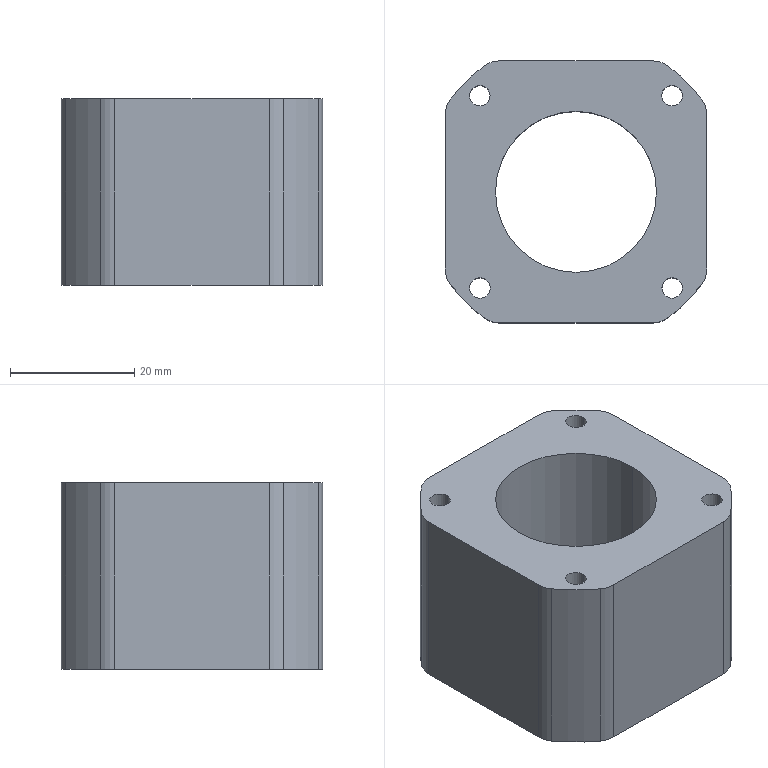Part | SolidWorks | features BaseBody 1 | 1 solid | 28 faces | box 42.13 x 42.13 x 30 mm | volume 33535 mm3 | cylinder 22 | plane 6 | commonest cylinder face diameters 3.3 x8 8 x8 50.215 x4 25.915 x2
STEP:
#1=CARTESIAN_POINT('',(-13.83,15.466,0.));
#2=VERTEX_POINT('',#1);
#3=CARTESIAN_POINT('',(-17.13,15.466,0.));
#4=VERTEX_POINT('',#3);
#5=CARTESIAN_POINT('',(-15.48,15.466,0.));
#6=DIRECTION('',(0.,0.,-1.));
#7=DIRECTION('',(1.,0.,0.));
#8=AXIS2_PLACEMENT_3D('',#5,#6,#7);
#9=CIRCLE('',#8,1.65);
#10=EDGE_CURVE('',#2,#4,#9,.T.);
#11=ORIENTED_EDGE('',*,*,#10,.T.);
#12=CARTESIAN_POINT('',(-17.13,15.466,30.));
#13=VERTEX_POINT('',#12);
#14=CARTESIAN_POINT('',(-17.13,15.466,0.));
#15=DIRECTION('',(0.,0.,1.));
#16=VECTOR('',#15,1000.);
#17=LINE('',#14,#16);
#18=EDGE_CURVE('',#4,#13,#17,.T.);
#19=ORIENTED_EDGE('',*,*,#18,.T.);
#20=CARTESIAN_POINT('',(-13.83,15.466,30.));
#21=VERTEX_POINT('',#20);
#22=CARTESIAN_POINT('',(-15.48,15.466,30.));
#23=DIRECTION('',(0.,0.,1.));
#24=DIRECTION('',(1.,0.,0.));
#25=AXIS2_PLACEMENT_3D('',#22,#23,#24);
#26=CIRCLE('',#25,1.65);
#27=EDGE_CURVE('',#13,#21,#26,.T.);
#28=ORIENTED_EDGE('',*,*,#27,.T.);
#29=CARTESIAN_POINT('',(-13.83,15.466,0.));
#30=DIRECTION('',(0.,0.,1.));
#31=VECTOR('',#30,1000.);
#32=LINE('',#29,#31);
#33=EDGE_CURVE('',#2,#21,#32,.T.);
#34=ORIENTED_EDGE('',*,*,#33,.F.);
#35=EDGE_LOOP('',(#11,#19,#28,#34));
#36=FACE_OUTER_BOUND('',#35,.T.);
#37=CARTESIAN_POINT('',(-15.48,15.466,0.));
#38=DIRECTION('',(0.,0.,1.));
#39=DIRECTION('',(1.,0.,0.));
#40=AXIS2_PLACEMENT_3D('',#37,#38,#39);
#41=CYLINDRICAL_SURFACE('',#40,1.65);
#42=ADVANCED_FACE('',(#36),#41,.F.);
#43=CARTESIAN_POINT('',(12.957,0.,0.));
#44=VERTEX_POINT('',#43);
#45=CARTESIAN_POINT('',(-12.957,0.,0.));
#46=VERTEX_POINT('',#45);
#47=CARTESIAN_POINT('',(0.,0.,0.));
#48=DIRECTION('',(0.,0.,-1.));
#49=DIRECTION('',(1.,0.,0.));
#50=AXIS2_PLACEMENT_3D('',#47,#48,#49);
#51=CIRCLE('',#50,12.957);
#52=EDGE_CURVE('',#44,#46,#51,.T.);
#53=ORIENTED_EDGE('',*,*,#52,.T.);
#54=CARTESIAN_POINT('',(-12.957,0.,30.));
#55=VERTEX_POINT('',#54);
#56=CARTESIAN_POINT('',(-12.957,0.,0.));
#57=DIRECTION('',(0.,0.,1.));
#58=VECTOR('',#57,1000.);
#59=LINE('',#56,#58);
#60=EDGE_CURVE('',#46,#55,#59,.T.);
#61=ORIENTED_EDGE('',*,*,#60,.T.);
#62=CARTESIAN_POINT('',(12.957,0.,30.));
#63=VERTEX_POINT('',#62);
#64=CARTESIAN_POINT('',(0.,0.,30.));
#65=DIRECTION('',(0.,0.,-1.));
#66=DIRECTION('',(1.,0.,0.));
#67=AXIS2_PLACEMENT_3D('',#64,#65,#66);
#68=CIRCLE('',#67,12.957);
#69=EDGE_CURVE('',#63,#55,#68,.T.);
#70=ORIENTED_EDGE('',*,*,#69,.F.);
#71=CARTESIAN_POINT('',(12.957,0.,0.));
#72=DIRECTION('',(0.,0.,1.));
#73=VECTOR('',#72,1000.);
#74=LINE('',#71,#73);
#75=EDGE_CURVE('',#44,#63,#74,.T.);
#76=ORIENTED_EDGE('',*,*,#75,.F.);
#77=EDGE_LOOP('',(#53,#61,#70,#76));
#78=FACE_OUTER_BOUND('',#77,.T.);
#79=CARTESIAN_POINT('',(0.,0.,0.));
#80=DIRECTION('',(0.,0.,1.));
#81=DIRECTION('',(1.,0.,0.));
#82=AXIS2_PLACEMENT_3D('',#79,#80,#81);
#83=CYLINDRICAL_SURFACE('',#82,12.957);
#84=ADVANCED_FACE('',(#78),#83,.F.);
#85=CARTESIAN_POINT('',(17.13,-15.466,0.));
#86=VERTEX_POINT('',#85);
#87=CARTESIAN_POINT('',(13.83,-15.466,0.));
#88=VERTEX_POINT('',#87);
#89=CARTESIAN_POINT('',(15.48,-15.466,0.));
#90=DIRECTION('',(0.,0.,-1.));
#91=DIRECTION('',(1.,0.,0.));
#92=AXIS2_PLACEMENT_3D('',#89,#90,#91);
#93=CIRCLE('',#92,1.65);
#94=EDGE_CURVE('',#86,#88,#93,.T.);
#95=ORIENTED_EDGE('',*,*,#94,.T.);
#96=CARTESIAN_POINT('',(13.83,-15.466,30.));
#97=VERTEX_POINT('',#96);
#98=CARTESIAN_POINT('',(13.83,-15.466,0.));
#99=DIRECTION('',(0.,0.,1.));
#100=VECTOR('',#99,1000.);
#101=LINE('',#98,#100);
#102=EDGE_CURVE('',#88,#97,#101,.T.);
#103=ORIENTED_EDGE('',*,*,#102,.T.);
#104=CARTESIAN_POINT('',(17.13,-15.466,30.));
#105=VERTEX_POINT('',#104);
#106=CARTESIAN_POINT('',(15.48,-15.466,30.));
#107=DIRECTION('',(0.,0.,-1.));
#108=DIRECTION('',(1.,0.,0.));
#109=AXIS2_PLACEMENT_3D('',#106,#107,#108);
#110=CIRCLE('',#109,1.65);
#111=EDGE_CURVE('',#105,#97,#110,.T.);
#112=ORIENTED_EDGE('',*,*,#111,.F.);
#113=CARTESIAN_POINT('',(17.13,-15.466,0.));
#114=DIRECTION('',(0.,0.,1.));
#115=VECTOR('',#114,1000.);
#116=LINE('',#113,#115);
#117=EDGE_CURVE('',#86,#105,#116,.T.);
#118=ORIENTED_EDGE('',*,*,#117,.F.);
#119=EDGE_LOOP('',(#95,#103,#112,#118));
#120=FACE_OUTER_BOUND('',#119,.T.);
#121=CARTESIAN_POINT('',(15.48,-15.466,0.));
#122=DIRECTION('',(0.,0.,1.));
#123=DIRECTION('',(1.,0.,0.));
#124=AXIS2_PLACEMENT_3D('',#121,#122,#123);
#125=CYLINDRICAL_SURFACE('',#124,1.65);
#126=ADVANCED_FACE('',(#120),#125,.F.);
#127=CARTESIAN_POINT('',(-13.816,-15.48,0.));
#128=VERTEX_POINT('',#127);
#129=CARTESIAN_POINT('',(-17.116,-15.48,0.));
#130=VERTEX_POINT('',#129);
#131=CARTESIAN_POINT('',(-15.466,-15.48,0.));
#132=DIRECTION('',(0.,0.,-1.));
#133=DIRECTION('',(1.,0.,0.));
#134=AXIS2_PLACEMENT_3D('',#131,#132,#133);
#135=CIRCLE('',#134,1.65);
#136=EDGE_CURVE('',#128,#130,#135,.T.);
#137=ORIENTED_EDGE('',*,*,#136,.T.);
#138=CARTESIAN_POINT('',(-17.116,-15.48,30.));
#139=VERTEX_POINT('',#138);
#140=CARTESIAN_POINT('',(-17.116,-15.48,0.));
#141=DIRECTION('',(0.,0.,1.));
#142=VECTOR('',#141,1000.);
#143=LINE('',#140,#142);
#144=EDGE_CURVE('',#130,#139,#143,.T.);
#145=ORIENTED_EDGE('',*,*,#144,.T.);
#146=CARTESIAN_POINT('',(-13.816,-15.48,30.));
#147=VERTEX_POINT('',#146);
#148=CARTESIAN_POINT('',(-15.466,-15.48,30.));
#149=DIRECTION('',(0.,0.,-1.));
#150=DIRECTION('',(1.,0.,0.));
#151=AXIS2_PLACEMENT_3D('',#148,#149,#150);
#152=CIRCLE('',#151,1.65);
#153=EDGE_CURVE('',#147,#139,#152,.T.);
#154=ORIENTED_EDGE('',*,*,#153,.F.);
#155=CARTESIAN_POINT('',(-13.816,-15.48,0.));
#156=DIRECTION('',(0.,0.,1.));
#157=VECTOR('',#156,1000.);
#158=LINE('',#155,#157);
#159=EDGE_CURVE('',#128,#147,#158,.T.);
#160=ORIENTED_EDGE('',*,*,#159,.F.);
#161=EDGE_LOOP('',(#137,#145,#154,#160));
#162=FACE_OUTER_BOUND('',#161,.T.);
#163=CARTESIAN_POINT('',(-15.466,-15.48,0.));
#164=DIRECTION('',(0.,0.,1.));
#165=DIRECTION('',(1.,0.,0.));
#166=AXIS2_PLACEMENT_3D('',#163,#164,#165);
#167=CYLINDRICAL_SURFACE('',#166,1.65);
#168=ADVANCED_FACE('',(#162),#167,.F.);
#169=CARTESIAN_POINT('',(17.116,15.48,0.));
#170=VERTEX_POINT('',#169);
#171=CARTESIAN_POINT('',(13.816,15.48,0.));
#172=VERTEX_POINT('',#171);
#173=CARTESIAN_POINT('',(15.466,15.48,0.));
#174=DIRECTION('',(0.,0.,-1.));
#175=DIRECTION('',(1.,0.,0.));
#176=AXIS2_PLACEMENT_3D('',#173,#174,#175);
#177=CIRCLE('',#176,1.65);
#178=EDGE_CURVE('',#170,#172,#177,.T.);
#179=ORIENTED_EDGE('',*,*,#178,.T.);
#180=CARTESIAN_POINT('',(13.816,15.48,30.));
#181=VERTEX_POINT('',#180);
#182=CARTESIAN_POINT('',(13.816,15.48,0.));
#183=DIRECTION('',(0.,0.,1.));
#184=VECTOR('',#183,1000.);
#185=LINE('',#182,#184);
#186=EDGE_CURVE('',#172,#181,#185,.T.);
#187=ORIENTED_EDGE('',*,*,#186,.T.);
#188=CARTESIAN_POINT('',(17.116,15.48,30.));
#189=VERTEX_POINT('',#188);
#190=CARTESIAN_POINT('',(15.466,15.48,30.));
#191=DIRECTION('',(0.,0.,-1.));
#192=DIRECTION('',(1.,0.,0.));
#193=AXIS2_PLACEMENT_3D('',#190,#191,#192);
#194=CIRCLE('',#193,1.65);
#195=EDGE_CURVE('',#189,#181,#194,.T.);
#196=ORIENTED_EDGE('',*,*,#195,.F.);
#197=CARTESIAN_POINT('',(17.116,15.48,0.));
#198=DIRECTION('',(0.,0.,1.));
#199=VECTOR('',#198,1000.);
#200=LINE('',#197,#199);
#201=EDGE_CURVE('',#170,#189,#200,.T.);
#202=ORIENTED_EDGE('',*,*,#201,.F.);
#203=EDGE_LOOP('',(#179,#187,#196,#202));
#204=FACE_OUTER_BOUND('',#203,.T.);
#205=CARTESIAN_POINT('',(15.466,15.48,0.));
#206=DIRECTION('',(0.,0.,1.));
#207=DIRECTION('',(1.,0.,0.));
#208=AXIS2_PLACEMENT_3D('',#205,#206,#207);
#209=CYLINDRICAL_SURFACE('',#208,1.65);
#210=ADVANCED_FACE('',(#204),#209,.F.);
#211=CARTESIAN_POINT('',(-14.776,20.299,0.));
#212=VERTEX_POINT('',#211);
#213=CARTESIAN_POINT('',(-14.776,20.299,30.));
#214=VERTEX_POINT('',#213);
#215=CARTESIAN_POINT('',(-14.776,20.299,15.));
#216=DIRECTION('',(0.,0.,1.));
#217=VECTOR('',#216,1000.);
#218=LINE('',#215,#217);
#219=EDGE_CURVE('',#212,#214,#218,.T.);
#220=ORIENTED_EDGE('',*,*,#219,.T.);
#221=CARTESIAN_POINT('',(-12.422,21.065,30.));
#222=VERTEX_POINT('',#221);
#223=CARTESIAN_POINT('',(-12.422,17.065,30.));
#224=DIRECTION('',(0.,0.,1.));
#225=DIRECTION('',(0.,1.,0.));
#226=AXIS2_PLACEMENT_3D('',#223,#224,#225);
#227=CIRCLE('',#226,4.);
#228=EDGE_CURVE('',#222,#214,#227,.T.);
#229=ORIENTED_EDGE('',*,*,#228,.F.);
#230=CARTESIAN_POINT('',(-12.422,21.065,0.));
#231=VERTEX_POINT('',#230);
#232=CARTESIAN_POINT('',(-12.422,21.065,15.));
#233=DIRECTION('',(0.,0.,-1.));
#234=VECTOR('',#233,1000.);
#235=LINE('',#232,#234);
#236=EDGE_CURVE('',#222,#231,#235,.T.);
#237=ORIENTED_EDGE('',*,*,#236,.T.);
#238=CARTESIAN_POINT('',(-12.422,17.065,0.));
#239=DIRECTION('',(0.,0.,1.));
#240=DIRECTION('',(0.,1.,0.));
#241=AXIS2_PLACEMENT_3D('',#238,#239,#240);
#242=CIRCLE('',#241,4.);
#243=EDGE_CURVE('',#231,#212,#242,.T.);
#244=ORIENTED_EDGE('',*,*,#243,.T.);
#245=EDGE_LOOP('',(#220,#229,#237,#244));
#246=FACE_OUTER_BOUND('',#245,.T.);
#247=CARTESIAN_POINT('',(-12.422,17.065,30.));
#248=DIRECTION('',(0.,0.,-1.));
#249=DIRECTION('',(0.,1.,0.));
#250=AXIS2_PLACEMENT_3D('',#247,#248,#249);
#251=CYLINDRICAL_SURFACE('',#250,4.);
#252=ADVANCED_FACE('',(#246),#251,.T.);
#253=CARTESIAN_POINT('',(-20.299,14.776,0.));
#254=VERTEX_POINT('',#253);
#255=CARTESIAN_POINT('',(-20.299,14.776,30.));
#256=VERTEX_POINT('',#255);
#257=CARTESIAN_POINT('',(-20.299,14.776,15.));
#258=DIRECTION('',(0.,0.,1.));
#259=VECTOR('',#258,1000.);
#260=LINE('',#257,#259);
#261=EDGE_CURVE('',#254,#256,#260,.T.);
#262=ORIENTED_EDGE('',*,*,#261,.T.);
#263=CARTESIAN_POINT('',(0.,0.,30.));
#264=DIRECTION('',(0.,0.,1.));
#265=DIRECTION('',(0.,1.,0.));
#266=AXIS2_PLACEMENT_3D('',#263,#264,#265);
#267=CIRCLE('',#266,25.108);
#268=EDGE_CURVE('',#214,#256,#267,.T.);
#269=ORIENTED_EDGE('',*,*,#268,.F.);
#270=ORIENTED_EDGE('',*,*,#219,.F.);
#271=CARTESIAN_POINT('',(0.,0.,0.));
#272=DIRECTION('',(0.,0.,1.));
#273=DIRECTION('',(0.,1.,0.));
#274=AXIS2_PLACEMENT_3D('',#271,#272,#273);
#275=CIRCLE('',#274,25.108);
#276=EDGE_CURVE('',#212,#254,#275,.T.);
#277=ORIENTED_EDGE('',*,*,#276,.T.);
#278=EDGE_LOOP('',(#262,#269,#270,#277));
#279=FACE_OUTER_BOUND('',#278,.T.);
#280=CARTESIAN_POINT('',(0.,0.,30.));
#281=DIRECTION('',(0.,0.,-1.));
#282=DIRECTION('',(0.,1.,0.));
#283=AXIS2_PLACEMENT_3D('',#280,#281,#282);
#284=CYLINDRICAL_SURFACE('',#283,25.108);
#285=ADVANCED_FACE('',(#279),#284,.T.);
#286=CARTESIAN_POINT('',(-21.065,12.422,0.));
#287=VERTEX_POINT('',#286);
#288=CARTESIAN_POINT('',(-21.065,12.422,30.));
#289=VERTEX_POINT('',#288);
#290=CARTESIAN_POINT('',(-21.065,12.422,15.));
#291=DIRECTION('',(0.,0.,1.));
#292=VECTOR('',#291,1000.);
#293=LINE('',#290,#292);
#294=EDGE_CURVE('',#287,#289,#293,.T.);
#295=ORIENTED_EDGE('',*,*,#294,.T.);
#296=CARTESIAN_POINT('',(-17.065,12.422,30.));
#297=DIRECTION('',(0.,0.,1.));
#298=DIRECTION('',(0.,1.,0.));
#299=AXIS2_PLACEMENT_3D('',#296,#297,#298);
#300=CIRCLE('',#299,4.);
#301=EDGE_CURVE('',#256,#289,#300,.T.);
#302=ORIENTED_EDGE('',*,*,#301,.F.);
#303=ORIENTED_EDGE('',*,*,#261,.F.);
#304=CARTESIAN_POINT('',(-17.065,12.422,0.));
#305=DIRECTION('',(0.,0.,1.));
#306=DIRECTION('',(0.,1.,0.));
#307=AXIS2_PLACEMENT_3D('',#304,#305,#306);
#308=CIRCLE('',#307,4.);
#309=EDGE_CURVE('',#254,#287,#308,.T.);
#310=ORIENTED_EDGE('',*,*,#309,.T.);
#311=EDGE_LOOP('',(#295,#302,#303,#310));
#312=FACE_OUTER_BOUND('',#311,.T.);
#313=CARTESIAN_POINT('',(-17.065,12.422,30.));
#314=DIRECTION('',(0.,0.,-1.));
#315=DIRECTION('',(0.,1.,0.));
#316=AXIS2_PLACEMENT_3D('',#313,#314,#315);
#317=CYLINDRICAL_SURFACE('',#316,4.);
#318=ADVANCED_FACE('',(#312),#317,.T.);
#319=CARTESIAN_POINT('',(-21.065,-12.422,0.));
#320=VERTEX_POINT('',#319);
#321=CARTESIAN_POINT('',(-21.065,-12.422,30.));
#322=VERTEX_POINT('',#321);
#323=CARTESIAN_POINT('',(-21.065,-12.422,15.));
#324=DIRECTION('',(0.,0.,1.));
#325=VECTOR('',#324,1000.);
#326=LINE('',#323,#325);
#327=EDGE_CURVE('',#320,#322,#326,.T.);
#328=ORIENTED_EDGE('',*,*,#327,.T.);
#329=CARTESIAN_POINT('',(-21.065,0.,30.));
#330=DIRECTION('',(0.,-1.,0.));
#331=VECTOR('',#330,1000.);
#332=LINE('',#329,#331);
#333=EDGE_CURVE('',#289,#322,#332,.T.);
#334=ORIENTED_EDGE('',*,*,#333,.F.);
#335=ORIENTED_EDGE('',*,*,#294,.F.);
#336=CARTESIAN_POINT('',(-21.065,0.,0.));
#337=DIRECTION('',(0.,-1.,0.));
#338=VECTOR('',#337,1000.);
#339=LINE('',#336,#338);
#340=EDGE_CURVE('',#287,#320,#339,.T.);
#341=ORIENTED_EDGE('',*,*,#340,.T.);
#342=EDGE_LOOP('',(#328,#334,#335,#341));
#343=FACE_OUTER_BOUND('',#342,.T.);
#344=CARTESIAN_POINT('',(-21.065,-12.422,30.));
#345=DIRECTION('',(1.,0.,0.));
#346=DIRECTION('',(0.,1.,0.));
#347=AXIS2_PLACEMENT_3D('',#344,#345,#346);
#348=PLANE('',#347);
#349=ADVANCED_FACE('',(#343),#348,.F.);
#350=CARTESIAN_POINT('',(-20.299,-14.776,0.));
#351=VERTEX_POINT('',#350);
#352=CARTESIAN_POINT('',(-20.299,-14.776,30.));
#353=VERTEX_POINT('',#352);
#354=CARTESIAN_POINT('',(-20.299,-14.776,15.));
#355=DIRECTION('',(0.,0.,1.));
#356=VECTOR('',#355,1000.);
#357=LINE('',#354,#356);
#358=EDGE_CURVE('',#351,#353,#357,.T.);
#359=ORIENTED_EDGE('',*,*,#358,.T.);
#360=CARTESIAN_POINT('',(-17.065,-12.422,30.));
#361=DIRECTION('',(0.,0.,1.));
#362=DIRECTION('',(0.,1.,0.));
#363=AXIS2_PLACEMENT_3D('',#360,#361,#362);
#364=CIRCLE('',#363,4.);
#365=EDGE_CURVE('',#322,#353,#364,.T.);
#366=ORIENTED_EDGE('',*,*,#365,.F.);
#367=ORIENTED_EDGE('',*,*,#327,.F.);
#368=CARTESIAN_POINT('',(-17.065,-12.422,0.));
#369=DIRECTION('',(0.,0.,1.));
#370=DIRECTION('',(0.,1.,0.));
#371=AXIS2_PLACEMENT_3D('',#368,#369,#370);
#372=CIRCLE('',#371,4.);
#373=EDGE_CURVE('',#320,#351,#372,.T.);
#374=ORIENTED_EDGE('',*,*,#373,.T.);
#375=EDGE_LOOP('',(#359,#366,#367,#374));
#376=FACE_OUTER_BOUND('',#375,.T.);
#377=CARTESIAN_POINT('',(-17.065,-12.422,30.));
#378=DIRECTION('',(0.,0.,-1.));
#379=DIRECTION('',(0.,1.,0.));
#380=AXIS2_PLACEMENT_3D('',#377,#378,#379);
#381=CYLINDRICAL_SURFACE('',#380,4.);
#382=ADVANCED_FACE('',(#376),#381,.T.);
#383=CARTESIAN_POINT('',(-14.776,-20.299,0.));
#384=VERTEX_POINT('',#383);
#385=CARTESIAN_POINT('',(-14.776,-20.299,30.));
#386=VERTEX_POINT('',#385);
#387=CARTESIAN_POINT('',(-14.776,-20.299,15.));
#388=DIRECTION('',(0.,0.,1.));
#389=VECTOR('',#388,1000.);
#390=LINE('',#387,#389);
#391=EDGE_CURVE('',#384,#386,#390,.T.);
#392=ORIENTED_EDGE('',*,*,#391,.T.);
#393=CARTESIAN_POINT('',(0.,0.,30.));
#394=DIRECTION('',(0.,0.,1.));
#395=DIRECTION('',(0.,1.,0.));
#396=AXIS2_PLACEMENT_3D('',#393,#394,#395);
#397=CIRCLE('',#396,25.108);
#398=EDGE_CURVE('',#353,#386,#397,.T.);
#399=ORIENTED_EDGE('',*,*,#398,.F.);
#400=ORIENTED_EDGE('',*,*,#358,.F.);
#401=CARTESIAN_POINT('',(0.,0.,0.));
#402=DIRECTION('',(0.,0.,1.));
#403=DIRECTION('',(0.,1.,0.));
#404=AXIS2_PLACEMENT_3D('',#401,#402,#403);
#405=CIRCLE('',#404,25.108);
#406=EDGE_CURVE('',#351,#384,#405,.T.);
#407=ORIENTED_EDGE('',*,*,#406,.T.);
#408=EDGE_LOOP('',(#392,#399,#400,#407));
#409=FACE_OUTER_BOUND('',#408,.T.);
#410=CARTESIAN_POINT('',(0.,0.,30.));
#411=DIRECTION('',(0.,0.,-1.));
#412=DIRECTION('',(0.,1.,0.));
#413=AXIS2_PLACEMENT_3D('',#410,#411,#412);
#414=CYLINDRICAL_SURFACE('',#413,25.108);
#415=ADVANCED_FACE('',(#409),#414,.T.);
#416=CARTESIAN_POINT('',(-12.422,-21.065,0.));
#417=VERTEX_POINT('',#416);
#418=CARTESIAN_POINT('',(-12.422,-21.065,30.));
#419=VERTEX_POINT('',#418);
#420=CARTESIAN_POINT('',(-12.422,-21.065,15.));
#421=DIRECTION('',(0.,0.,1.));
#422=VECTOR('',#421,1000.);
#423=LINE('',#420,#422);
#424=EDGE_CURVE('',#417,#419,#423,.T.);
#425=ORIENTED_EDGE('',*,*,#424,.T.);
#426=CARTESIAN_POINT('',(-12.422,-17.065,30.));
#427=DIRECTION('',(0.,0.,1.));
#428=DIRECTION('',(0.,1.,0.));
#429=AXIS2_PLACEMENT_3D('',#426,#427,#428);
#430=CIRCLE('',#429,4.);
#431=EDGE_CURVE('',#386,#419,#430,.T.);
#432=ORIENTED_EDGE('',*,*,#431,.F.);
#433=ORIENTED_EDGE('',*,*,#391,.F.);
#434=CARTESIAN_POINT('',(-12.422,-17.065,0.));
#435=DIRECTION('',(0.,0.,1.));
#436=DIRECTION('',(0.,1.,0.));
#437=AXIS2_PLACEMENT_3D('',#434,#435,#436);
#438=CIRCLE('',#437,4.);
#439=EDGE_CURVE('',#384,#417,#438,.T.);
#440=ORIENTED_EDGE('',*,*,#439,.T.);
#441=EDGE_LOOP('',(#425,#432,#433,#440));
#442=FACE_OUTER_BOUND('',#441,.T.);
#443=CARTESIAN_POINT('',(-12.422,-17.065,30.));
#444=DIRECTION('',(0.,0.,-1.));
#445=DIRECTION('',(0.,1.,0.));
#446=AXIS2_PLACEMENT_3D('',#443,#444,#445);
#447=CYLINDRICAL_SURFACE('',#446,4.);
#448=ADVANCED_FACE('',(#442),#447,.T.);
#449=CARTESIAN_POINT('',(12.422,-21.065,0.));
#450=VERTEX_POINT('',#449);
#451=CARTESIAN_POINT('',(12.422,-21.065,30.));
#452=VERTEX_POINT('',#451);
#453=CARTESIAN_POINT('',(12.422,-21.065,15.));
#454=DIRECTION('',(0.,0.,1.));
#455=VECTOR('',#454,1000.);
#456=LINE('',#453,#455);
#457=EDGE_CURVE('',#450,#452,#456,.T.);
#458=ORIENTED_EDGE('',*,*,#457,.T.);
#459=CARTESIAN_POINT('',(0.,-21.065,30.));
#460=DIRECTION('',(1.,0.,0.));
#461=VECTOR('',#460,1000.);
#462=LINE('',#459,#461);
#463=EDGE_CURVE('',#419,#452,#462,.T.);
#464=ORIENTED_EDGE('',*,*,#463,.F.);
#465=ORIENTED_EDGE('',*,*,#424,.F.);
#466=CARTESIAN_POINT('',(0.,-21.065,0.));
#467=DIRECTION('',(1.,0.,0.));
#468=VECTOR('',#467,1000.);
#469=LINE('',#466,#468);
#470=EDGE_CURVE('',#417,#450,#469,.T.);
#471=ORIENTED_EDGE('',*,*,#470,.T.);
#472=EDGE_LOOP('',(#458,#464,#465,#471));
#473=FACE_OUTER_BOUND('',#472,.T.);
#474=CARTESIAN_POINT('',(-12.422,-21.065,0.));
#475=DIRECTION('',(0.,1.,0.));
#476=DIRECTION('',(1.,0.,0.));
#477=AXIS2_PLACEMENT_3D('',#474,#475,#476);
#478=PLANE('',#477);
#479=ADVANCED_FACE('',(#473),#478,.F.);
#480=CARTESIAN_POINT('',(14.776,-20.299,0.));
#481=VERTEX_POINT('',#480);
#482=CARTESIAN_POINT('',(14.776,-20.299,30.));
#483=VERTEX_POINT('',#482);
#484=CARTESIAN_POINT('',(14.776,-20.299,15.));
#485=DIRECTION('',(0.,0.,1.));
#486=VECTOR('',#485,1000.);
#487=LINE('',#484,#486);
#488=EDGE_CURVE('',#481,#483,#487,.T.);
#489=ORIENTED_EDGE('',*,*,#488,.T.);
#490=CARTESIAN_POINT('',(12.422,-17.065,30.));
#491=DIRECTION('',(0.,0.,1.));
#492=DIRECTION('',(0.,1.,0.));
#493=AXIS2_PLACEMENT_3D('',#490,#491,#492);
#494=CIRCLE('',#493,4.);
#495=EDGE_CURVE('',#452,#483,#494,.T.);
#496=ORIENTED_EDGE('',*,*,#495,.F.);
#497=ORIENTED_EDGE('',*,*,#457,.F.);
#498=CARTESIAN_POINT('',(12.422,-17.065,0.));
#499=DIRECTION('',(0.,0.,1.));
#500=DIRECTION('',(0.,1.,0.));
#501=AXIS2_PLACEMENT_3D('',#498,#499,#500);
#502=CIRCLE('',#501,4.);
#503=EDGE_CURVE('',#450,#481,#502,.T.);
#504=ORIENTED_EDGE('',*,*,#503,.T.);
#505=EDGE_LOOP('',(#489,#496,#497,#504));
#506=FACE_OUTER_BOUND('',#505,.T.);
#507=CARTESIAN_POINT('',(12.422,-17.065,30.));
#508=DIRECTION('',(0.,0.,-1.));
#509=DIRECTION('',(0.,1.,0.));
#510=AXIS2_PLACEMENT_3D('',#507,#508,#509);
#511=CYLINDRICAL_SURFACE('',#510,4.);
#512=ADVANCED_FACE('',(#506),#511,.T.);
#513=CARTESIAN_POINT('',(20.299,-14.776,0.));
#514=VERTEX_POINT('',#513);
#515=CARTESIAN_POINT('',(20.299,-14.776,30.));
#516=VERTEX_POINT('',#515);
#517=CARTESIAN_POINT('',(20.299,-14.776,15.));
#518=DIRECTION('',(0.,0.,1.));
#519=VECTOR('',#518,1000.);
#520=LINE('',#517,#519);
#521=EDGE_CURVE('',#514,#516,#520,.T.);
#522=ORIENTED_EDGE('',*,*,#521,.T.);
#523=CARTESIAN_POINT('',(0.,0.,30.));
#524=DIRECTION('',(0.,0.,1.));
#525=DIRECTION('',(0.,1.,0.));
#526=AXIS2_PLACEMENT_3D('',#523,#524,#525);
#527=CIRCLE('',#526,25.108);
#528=EDGE_CURVE('',#483,#516,#527,.T.);
#529=ORIENTED_EDGE('',*,*,#528,.F.);
#530=ORIENTED_EDGE('',*,*,#488,.F.);
#531=CARTESIAN_POINT('',(0.,0.,0.));
#532=DIRECTION('',(0.,0.,1.));
#533=DIRECTION('',(0.,1.,0.));
#534=AXIS2_PLACEMENT_3D('',#531,#532,#533);
#535=CIRCLE('',#534,25.108);
#536=EDGE_CURVE('',#481,#514,#535,.T.);
#537=ORIENTED_EDGE('',*,*,#536,.T.);
#538=EDGE_LOOP('',(#522,#529,#530,#537));
#539=FACE_OUTER_BOUND('',#538,.T.);
#540=CARTESIAN_POINT('',(0.,0.,30.));
#541=DIRECTION('',(0.,0.,-1.));
#542=DIRECTION('',(0.,1.,0.));
#543=AXIS2_PLACEMENT_3D('',#540,#541,#542);
#544=CYLINDRICAL_SURFACE('',#543,25.108);
#545=ADVANCED_FACE('',(#539),#544,.T.);
#546=CARTESIAN_POINT('',(21.065,-12.422,0.));
#547=VERTEX_POINT('',#546);
#548=CARTESIAN_POINT('',(21.065,-12.422,30.));
#549=VERTEX_POINT('',#548);
#550=CARTESIAN_POINT('',(21.065,-12.422,15.));
#551=DIRECTION('',(0.,0.,1.));
#552=VECTOR('',#551,1000.);
#553=LINE('',#550,#552);
#554=EDGE_CURVE('',#547,#549,#553,.T.);
#555=ORIENTED_EDGE('',*,*,#554,.T.);
#556=CARTESIAN_POINT('',(17.065,-12.422,30.));
#557=DIRECTION('',(0.,0.,1.));
#558=DIRECTION('',(0.,1.,0.));
#559=AXIS2_PLACEMENT_3D('',#556,#557,#558);
#560=CIRCLE('',#559,4.);
#561=EDGE_CURVE('',#516,#549,#560,.T.);
#562=ORIENTED_EDGE('',*,*,#561,.F.);
#563=ORIENTED_EDGE('',*,*,#521,.F.);
#564=CARTESIAN_POINT('',(17.065,-12.422,0.));
#565=DIRECTION('',(0.,0.,1.));
#566=DIRECTION('',(0.,1.,0.));
#567=AXIS2_PLACEMENT_3D('',#564,#565,#566);
#568=CIRCLE('',#567,4.);
#569=EDGE_CURVE('',#514,#547,#568,.T.);
#570=ORIENTED_EDGE('',*,*,#569,.T.);
#571=EDGE_LOOP('',(#555,#562,#563,#570));
#572=FACE_OUTER_BOUND('',#571,.T.);
#573=CARTESIAN_POINT('',(17.065,-12.422,30.));
#574=DIRECTION('',(0.,0.,-1.));
#575=DIRECTION('',(0.,1.,0.));
#576=AXIS2_PLACEMENT_3D('',#573,#574,#575);
#577=CYLINDRICAL_SURFACE('',#576,4.);
#578=ADVANCED_FACE('',(#572),#577,.T.);
#579=CARTESIAN_POINT('',(21.065,12.422,0.));
#580=VERTEX_POINT('',#579);
#581=CARTESIAN_POINT('',(21.065,12.422,30.));
#582=VERTEX_POINT('',#581);
#583=CARTESIAN_POINT('',(21.065,12.422,15.));
#584=DIRECTION('',(0.,0.,1.));
#585=VECTOR('',#584,1000.);
#586=LINE('',#583,#585);
#587=EDGE_CURVE('',#580,#582,#586,.T.);
#588=ORIENTED_EDGE('',*,*,#587,.T.);
#589=CARTESIAN_POINT('',(21.065,0.,30.));
#590=DIRECTION('',(0.,1.,0.));
#591=VECTOR('',#590,1000.);
#592=LINE('',#589,#591);
#593=EDGE_CURVE('',#549,#582,#592,.T.);
#594=ORIENTED_EDGE('',*,*,#593,.F.);
#595=ORIENTED_EDGE('',*,*,#554,.F.);
#596=CARTESIAN_POINT('',(21.065,0.,0.));
#597=DIRECTION('',(0.,1.,0.));
#598=VECTOR('',#597,1000.);
#599=LINE('',#596,#598);
#600=EDGE_CURVE('',#547,#580,#599,.T.);
#601=ORIENTED_EDGE('',*,*,#600,.T.);
#602=EDGE_LOOP('',(#588,#594,#595,#601));
#603=FACE_OUTER_BOUND('',#602,.T.);
#604=CARTESIAN_POINT('',(21.065,-12.422,0.));
#605=DIRECTION('',(-1.,0.,0.));
#606=DIRECTION('',(0.,0.,1.));
#607=AXIS2_PLACEMENT_3D('',#604,#605,#606);
#608=PLANE('',#607);
#609=ADVANCED_FACE('',(#603),#608,.F.);
#610=CARTESIAN_POINT('',(20.299,14.776,0.));
#611=VERTEX_POINT('',#610);
#612=CARTESIAN_POINT('',(20.299,14.776,30.));
#613=VERTEX_POINT('',#612);
#614=CARTESIAN_POINT('',(20.299,14.776,15.));
#615=DIRECTION('',(0.,0.,1.));
#616=VECTOR('',#615,1000.);
#617=LINE('',#614,#616);
#618=EDGE_CURVE('',#611,#613,#617,.T.);
#619=ORIENTED_EDGE('',*,*,#618,.T.);
#620=CARTESIAN_POINT('',(17.065,12.422,30.));
#621=DIRECTION('',(0.,0.,1.));
#622=DIRECTION('',(0.,1.,0.));
#623=AXIS2_PLACEMENT_3D('',#620,#621,#622);
#624=CIRCLE('',#623,4.);
#625=EDGE_CURVE('',#582,#613,#624,.T.);
#626=ORIENTED_EDGE('',*,*,#625,.F.);
#627=ORIENTED_EDGE('',*,*,#587,.F.);
#628=CARTESIAN_POINT('',(17.065,12.422,0.));
#629=DIRECTION('',(0.,0.,1.));
#630=DIRECTION('',(0.,1.,0.));
#631=AXIS2_PLACEMENT_3D('',#628,#629,#630);
#632=CIRCLE('',#631,4.);
#633=EDGE_CURVE('',#580,#611,#632,.T.);
#634=ORIENTED_EDGE('',*,*,#633,.T.);
#635=EDGE_LOOP('',(#619,#626,#627,#634));
#636=FACE_OUTER_BOUND('',#635,.T.);
#637=CARTESIAN_POINT('',(17.065,12.422,30.));
#638=DIRECTION('',(0.,0.,-1.));
#639=DIRECTION('',(0.,1.,0.));
#640=AXIS2_PLACEMENT_3D('',#637,#638,#639);
#641=CYLINDRICAL_SURFACE('',#640,4.);
#642=ADVANCED_FACE('',(#636),#641,.T.);
#643=CARTESIAN_POINT('',(14.776,20.299,0.));
#644=VERTEX_POINT('',#643);
#645=CARTESIAN_POINT('',(14.776,20.299,30.));
#646=VERTEX_POINT('',#645);
#647=CARTESIAN_POINT('',(14.776,20.299,15.));
#648=DIRECTION('',(0.,0.,1.));
#649=VECTOR('',#648,1000.);
#650=LINE('',#647,#649);
#651=EDGE_CURVE('',#644,#646,#650,.T.);
#652=ORIENTED_EDGE('',*,*,#651,.T.);
#653=CARTESIAN_POINT('',(0.,0.,30.));
#654=DIRECTION('',(0.,0.,1.));
#655=DIRECTION('',(0.,1.,0.));
#656=AXIS2_PLACEMENT_3D('',#653,#654,#655);
#657=CIRCLE('',#656,25.108);
#658=EDGE_CURVE('',#613,#646,#657,.T.);
#659=ORIENTED_EDGE('',*,*,#658,.F.);
#660=ORIENTED_EDGE('',*,*,#618,.F.);
#661=CARTESIAN_POINT('',(0.,0.,0.));
#662=DIRECTION('',(0.,0.,1.));
#663=DIRECTION('',(0.,1.,0.));
#664=AXIS2_PLACEMENT_3D('',#661,#662,#663);
#665=CIRCLE('',#664,25.108);
#666=EDGE_CURVE('',#611,#644,#665,.T.);
#667=ORIENTED_EDGE('',*,*,#666,.T.);
#668=EDGE_LOOP('',(#652,#659,#660,#667));
#669=FACE_OUTER_BOUND('',#668,.T.);
#670=CARTESIAN_POINT('',(0.,0.,30.));
#671=DIRECTION('',(0.,0.,-1.));
#672=DIRECTION('',(0.,1.,0.));
#673=AXIS2_PLACEMENT_3D('',#670,#671,#672);
#674=CYLINDRICAL_SURFACE('',#673,25.108);
#675=ADVANCED_FACE('',(#669),#674,.T.);
#676=CARTESIAN_POINT('',(12.422,21.065,0.));
#677=VERTEX_POINT('',#676);
#678=CARTESIAN_POINT('',(12.422,21.065,30.));
#679=VERTEX_POINT('',#678);
#680=CARTESIAN_POINT('',(12.422,21.065,15.));
#681=DIRECTION('',(0.,0.,1.));
#682=VECTOR('',#681,1000.);
#683=LINE('',#680,#682);
#684=EDGE_CURVE('',#677,#679,#683,.T.);
#685=ORIENTED_EDGE('',*,*,#684,.T.);
#686=CARTESIAN_POINT('',(12.422,17.065,30.));
#687=DIRECTION('',(0.,0.,1.));
#688=DIRECTION('',(0.,1.,0.));
#689=AXIS2_PLACEMENT_3D('',#686,#687,#688);
#690=CIRCLE('',#689,4.);
#691=EDGE_CURVE('',#646,#679,#690,.T.);
#692=ORIENTED_EDGE('',*,*,#691,.F.);
#693=ORIENTED_EDGE('',*,*,#651,.F.);
#694=CARTESIAN_POINT('',(12.422,17.065,0.));
#695=DIRECTION('',(0.,0.,1.));
#696=DIRECTION('',(0.,1.,0.));
#697=AXIS2_PLACEMENT_3D('',#694,#695,#696);
#698=CIRCLE('',#697,4.);
#699=EDGE_CURVE('',#644,#677,#698,.T.);
#700=ORIENTED_EDGE('',*,*,#699,.T.);
#701=EDGE_LOOP('',(#685,#692,#693,#700));
#702=FACE_OUTER_BOUND('',#701,.T.);
#703=CARTESIAN_POINT('',(12.422,17.065,30.));
#704=DIRECTION('',(0.,0.,-1.));
#705=DIRECTION('',(0.,1.,0.));
#706=AXIS2_PLACEMENT_3D('',#703,#704,#705);
#707=CYLINDRICAL_SURFACE('',#706,4.);
#708=ADVANCED_FACE('',(#702),#707,.T.);
#709=ORIENTED_EDGE('',*,*,#236,.F.);
#710=CARTESIAN_POINT('',(0.,21.065,30.));
#711=DIRECTION('',(-1.,0.,0.));
#712=VECTOR('',#711,1000.);
#713=LINE('',#710,#712);
#714=EDGE_CURVE('',#679,#222,#713,.T.);
#715=ORIENTED_EDGE('',*,*,#714,.F.);
#716=ORIENTED_EDGE('',*,*,#684,.F.);
#717=CARTESIAN_POINT('',(0.,21.065,0.));
#718=DIRECTION('',(-1.,0.,0.));
#719=VECTOR('',#718,1000.);
#720=LINE('',#717,#719);
#721=EDGE_CURVE('',#677,#231,#720,.T.);
#722=ORIENTED_EDGE('',*,*,#721,.T.);
#723=EDGE_LOOP('',(#709,#715,#716,#722));
#724=FACE_OUTER_BOUND('',#723,.T.);
#725=CARTESIAN_POINT('',(-12.422,21.065,30.));
#726=DIRECTION('',(0.,-1.,0.));
#727=DIRECTION('',(0.,0.,-1.));
#728=AXIS2_PLACEMENT_3D('',#725,#726,#727);
#729=PLANE('',#728);
#730=ADVANCED_FACE('',(#724),#729,.F.);
#731=ORIENTED_EDGE('',*,*,#186,.F.);
#732=CARTESIAN_POINT('',(15.466,15.48,0.));
#733=DIRECTION('',(0.,0.,-1.));
#734=DIRECTION('',(1.,0.,0.));
#735=AXIS2_PLACEMENT_3D('',#732,#733,#734);
#736=CIRCLE('',#735,1.65);
#737=EDGE_CURVE('',#172,#170,#736,.T.);
#738=ORIENTED_EDGE('',*,*,#737,.T.);
#739=ORIENTED_EDGE('',*,*,#201,.T.);
#740=CARTESIAN_POINT('',(15.466,15.48,30.));
#741=DIRECTION('',(0.,0.,-1.));
#742=DIRECTION('',(1.,0.,0.));
#743=AXIS2_PLACEMENT_3D('',#740,#741,#742);
#744=CIRCLE('',#743,1.65);
#745=EDGE_CURVE('',#181,#189,#744,.T.);
#746=ORIENTED_EDGE('',*,*,#745,.F.);
#747=EDGE_LOOP('',(#731,#738,#739,#746));
#748=FACE_OUTER_BOUND('',#747,.T.);
#749=CARTESIAN_POINT('',(15.466,15.48,0.));
#750=DIRECTION('',(0.,0.,1.));
#751=DIRECTION('',(1.,0.,0.));
#752=AXIS2_PLACEMENT_3D('',#749,#750,#751);
#753=CYLINDRICAL_SURFACE('',#752,1.65);
#754=ADVANCED_FACE('',(#748),#753,.F.);
#755=ORIENTED_EDGE('',*,*,#144,.F.);
#756=CARTESIAN_POINT('',(-15.466,-15.48,0.));
#757=DIRECTION('',(0.,0.,-1.));
#758=DIRECTION('',(1.,0.,0.));
#759=AXIS2_PLACEMENT_3D('',#756,#757,#758);
#760=CIRCLE('',#759,1.65);
#761=EDGE_CURVE('',#130,#128,#760,.T.);
#762=ORIENTED_EDGE('',*,*,#761,.T.);
#763=ORIENTED_EDGE('',*,*,#159,.T.);
#764=CARTESIAN_POINT('',(-15.466,-15.48,30.));
#765=DIRECTION('',(0.,0.,-1.));
#766=DIRECTION('',(1.,0.,0.));
#767=AXIS2_PLACEMENT_3D('',#764,#765,#766);
#768=CIRCLE('',#767,1.65);
#769=EDGE_CURVE('',#139,#147,#768,.T.);
#770=ORIENTED_EDGE('',*,*,#769,.F.);
#771=EDGE_LOOP('',(#755,#762,#763,#770));
#772=FACE_OUTER_BOUND('',#771,.T.);
#773=CARTESIAN_POINT('',(-15.466,-15.48,0.));
#774=DIRECTION('',(0.,0.,1.));
#775=DIRECTION('',(1.,0.,0.));
#776=AXIS2_PLACEMENT_3D('',#773,#774,#775);
#777=CYLINDRICAL_SURFACE('',#776,1.65);
#778=ADVANCED_FACE('',(#772),#777,.F.);
#779=ORIENTED_EDGE('',*,*,#102,.F.);
#780=CARTESIAN_POINT('',(15.48,-15.466,0.));
#781=DIRECTION('',(0.,0.,-1.));
#782=DIRECTION('',(1.,0.,0.));
#783=AXIS2_PLACEMENT_3D('',#780,#781,#782);
#784=CIRCLE('',#783,1.65);
#785=EDGE_CURVE('',#88,#86,#784,.T.);
#786=ORIENTED_EDGE('',*,*,#785,.T.);
#787=ORIENTED_EDGE('',*,*,#117,.T.);
#788=CARTESIAN_POINT('',(15.48,-15.466,30.));
#789=DIRECTION('',(0.,0.,-1.));
#790=DIRECTION('',(1.,0.,0.));
#791=AXIS2_PLACEMENT_3D('',#788,#789,#790);
#792=CIRCLE('',#791,1.65);
#793=EDGE_CURVE('',#97,#105,#792,.T.);
#794=ORIENTED_EDGE('',*,*,#793,.F.);
#795=EDGE_LOOP('',(#779,#786,#787,#794));
#796=FACE_OUTER_BOUND('',#795,.T.);
#797=CARTESIAN_POINT('',(15.48,-15.466,0.));
#798=DIRECTION('',(0.,0.,1.));
#799=DIRECTION('',(1.,0.,0.));
#800=AXIS2_PLACEMENT_3D('',#797,#798,#799);
#801=CYLINDRICAL_SURFACE('',#800,1.65);
#802=ADVANCED_FACE('',(#796),#801,.F.);
#803=ORIENTED_EDGE('',*,*,#60,.F.);
#804=CARTESIAN_POINT('',(0.,0.,0.));
#805=DIRECTION('',(0.,0.,-1.));
#806=DIRECTION('',(1.,0.,0.));
#807=AXIS2_PLACEMENT_3D('',#804,#805,#806);
#808=CIRCLE('',#807,12.957);
#809=EDGE_CURVE('',#46,#44,#808,.T.);
#810=ORIENTED_EDGE('',*,*,#809,.T.);
#811=ORIENTED_EDGE('',*,*,#75,.T.);
#812=CARTESIAN_POINT('',(0.,0.,30.));
#813=DIRECTION('',(0.,0.,-1.));
#814=DIRECTION('',(1.,0.,0.));
#815=AXIS2_PLACEMENT_3D('',#812,#813,#814);
#816=CIRCLE('',#815,12.957);
#817=EDGE_CURVE('',#55,#63,#816,.T.);
#818=ORIENTED_EDGE('',*,*,#817,.F.);
#819=EDGE_LOOP('',(#803,#810,#811,#818));
#820=FACE_OUTER_BOUND('',#819,.T.);
#821=CARTESIAN_POINT('',(0.,0.,0.));
#822=DIRECTION('',(0.,0.,1.));
#823=DIRECTION('',(1.,0.,0.));
#824=AXIS2_PLACEMENT_3D('',#821,#822,#823);
#825=CYLINDRICAL_SURFACE('',#824,12.957);
#826=ADVANCED_FACE('',(#820),#825,.F.);
#827=ORIENTED_EDGE('',*,*,#52,.F.);
#828=ORIENTED_EDGE('',*,*,#809,.F.);
#829=EDGE_LOOP('',(#827,#828));
#830=FACE_BOUND('',#829,.T.);
#831=ORIENTED_EDGE('',*,*,#94,.F.);
#832=ORIENTED_EDGE('',*,*,#785,.F.);
#833=EDGE_LOOP('',(#831,#832));
#834=FACE_BOUND('',#833,.T.);
#835=ORIENTED_EDGE('',*,*,#136,.F.);
#836=ORIENTED_EDGE('',*,*,#761,.F.);
#837=EDGE_LOOP('',(#835,#836));
#838=FACE_BOUND('',#837,.T.);
#839=ORIENTED_EDGE('',*,*,#178,.F.);
#840=ORIENTED_EDGE('',*,*,#737,.F.);
#841=EDGE_LOOP('',(#839,#840));
#842=FACE_BOUND('',#841,.T.);
#843=ORIENTED_EDGE('',*,*,#10,.F.);
#844=CARTESIAN_POINT('',(-15.48,15.466,0.));
#845=DIRECTION('',(0.,0.,-1.));
#846=DIRECTION('',(1.,0.,0.));
#847=AXIS2_PLACEMENT_3D('',#844,#845,#846);
#848=CIRCLE('',#847,1.65);
#849=EDGE_CURVE('',#4,#2,#848,.T.);
#850=ORIENTED_EDGE('',*,*,#849,.F.);
#851=EDGE_LOOP('',(#843,#850));
#852=FACE_BOUND('',#851,.T.);
#853=ORIENTED_EDGE('',*,*,#721,.F.);
#854=ORIENTED_EDGE('',*,*,#699,.F.);
#855=ORIENTED_EDGE('',*,*,#666,.F.);
#856=ORIENTED_EDGE('',*,*,#633,.F.);
#857=ORIENTED_EDGE('',*,*,#600,.F.);
#858=ORIENTED_EDGE('',*,*,#569,.F.);
#859=ORIENTED_EDGE('',*,*,#536,.F.);
#860=ORIENTED_EDGE('',*,*,#503,.F.);
#861=ORIENTED_EDGE('',*,*,#470,.F.);
#862=ORIENTED_EDGE('',*,*,#439,.F.);
#863=ORIENTED_EDGE('',*,*,#406,.F.);
#864=ORIENTED_EDGE('',*,*,#373,.F.);
#865=ORIENTED_EDGE('',*,*,#340,.F.);
#866=ORIENTED_EDGE('',*,*,#309,.F.);
#867=ORIENTED_EDGE('',*,*,#276,.F.);
#868=ORIENTED_EDGE('',*,*,#243,.F.);
#869=EDGE_LOOP('',(#853,#854,#855,#856,#857,#858,#859,#860,#861,#862,#863,#864,#865,#866,#867,#868));
#870=FACE_OUTER_BOUND('',#869,.T.);
#871=CARTESIAN_POINT('',(-21.065,-21.065,0.));
#872=DIRECTION('',(0.,0.,1.));
#873=DIRECTION('',(1.,0.,0.));
#874=AXIS2_PLACEMENT_3D('',#871,#872,#873);
#875=PLANE('',#874);
#876=ADVANCED_FACE('',(#830,#834,#838,#842,#852,#870),#875,.F.);
#877=ORIENTED_EDGE('',*,*,#69,.T.);
#878=ORIENTED_EDGE('',*,*,#817,.T.);
#879=EDGE_LOOP('',(#877,#878));
#880=FACE_BOUND('',#879,.T.);
#881=ORIENTED_EDGE('',*,*,#111,.T.);
#882=ORIENTED_EDGE('',*,*,#793,.T.);
#883=EDGE_LOOP('',(#881,#882));
#884=FACE_BOUND('',#883,.T.);
#885=ORIENTED_EDGE('',*,*,#153,.T.);
#886=ORIENTED_EDGE('',*,*,#769,.T.);
#887=EDGE_LOOP('',(#885,#886));
#888=FACE_BOUND('',#887,.T.);
#889=ORIENTED_EDGE('',*,*,#195,.T.);
#890=ORIENTED_EDGE('',*,*,#745,.T.);
#891=EDGE_LOOP('',(#889,#890));
#892=FACE_BOUND('',#891,.T.);
#893=CARTESIAN_POINT('',(-15.48,15.466,30.));
#894=DIRECTION('',(0.,0.,1.));
#895=DIRECTION('',(1.,0.,0.));
#896=AXIS2_PLACEMENT_3D('',#893,#894,#895);
#897=CIRCLE('',#896,1.65);
#898=EDGE_CURVE('',#21,#13,#897,.T.);
#899=ORIENTED_EDGE('',*,*,#898,.F.);
#900=ORIENTED_EDGE('',*,*,#27,.F.);
#901=EDGE_LOOP('',(#899,#900));
#902=FACE_BOUND('',#901,.T.);
#903=ORIENTED_EDGE('',*,*,#691,.T.);
#904=ORIENTED_EDGE('',*,*,#714,.T.);
#905=ORIENTED_EDGE('',*,*,#228,.T.);
#906=ORIENTED_EDGE('',*,*,#268,.T.);
#907=ORIENTED_EDGE('',*,*,#301,.T.);
#908=ORIENTED_EDGE('',*,*,#333,.T.);
#909=ORIENTED_EDGE('',*,*,#365,.T.);
#910=ORIENTED_EDGE('',*,*,#398,.T.);
#911=ORIENTED_EDGE('',*,*,#431,.T.);
#912=ORIENTED_EDGE('',*,*,#463,.T.);
#913=ORIENTED_EDGE('',*,*,#495,.T.);
#914=ORIENTED_EDGE('',*,*,#528,.T.);
#915=ORIENTED_EDGE('',*,*,#561,.T.);
#916=ORIENTED_EDGE('',*,*,#593,.T.);
#917=ORIENTED_EDGE('',*,*,#625,.T.);
#918=ORIENTED_EDGE('',*,*,#658,.T.);
#919=EDGE_LOOP('',(#903,#904,#905,#906,#907,#908,#909,#910,#911,#912,#913,#914,#915,#916,#917,#918));
#920=FACE_OUTER_BOUND('',#919,.T.);
#921=CARTESIAN_POINT('',(-21.065,-21.065,30.));
#922=DIRECTION('',(0.,0.,1.));
#923=DIRECTION('',(1.,0.,0.));
#924=AXIS2_PLACEMENT_3D('',#921,#922,#923);
#925=PLANE('',#924);
#926=ADVANCED_FACE('',(#880,#884,#888,#892,#902,#920),#925,.T.);
#927=ORIENTED_EDGE('',*,*,#18,.F.);
#928=ORIENTED_EDGE('',*,*,#849,.T.);
#929=ORIENTED_EDGE('',*,*,#33,.T.);
#930=ORIENTED_EDGE('',*,*,#898,.T.);
#931=EDGE_LOOP('',(#927,#928,#929,#930));
#932=FACE_OUTER_BOUND('',#931,.T.);
#933=CARTESIAN_POINT('',(-15.48,15.466,0.));
#934=DIRECTION('',(0.,0.,1.));
#935=DIRECTION('',(1.,0.,0.));
#936=AXIS2_PLACEMENT_3D('',#933,#934,#935);
#937=CYLINDRICAL_SURFACE('',#936,1.65);
#938=ADVANCED_FACE('',(#932),#937,.F.);
#939=CLOSED_SHELL('',(#42,#84,#126,#168,#210,#252,#285,#318,#349,#382,#415,#448,#479,#512,#545,#578,#609,#642,#675,#708,#730,#754,#778,#802,#826,#876,#926,#938));
#940=MANIFOLD_SOLID_BREP('',#939);
#941=CARTESIAN_POINT('',(0.,0.,0.));
#942=DIRECTION('',(0.,0.,1.));
#943=DIRECTION('',(1.,0.,0.));
#944=AXIS2_PLACEMENT_3D('',#941,#942,#943);
#945=(LENGTH_UNIT()NAMED_UNIT(*)SI_UNIT(.MILLI.,.METRE.));
#946=UNCERTAINTY_MEASURE_WITH_UNIT(LENGTH_MEASURE(0.00001),#945,'','');
#947=(NAMED_UNIT(*)PLANE_ANGLE_UNIT()SI_UNIT($,.RADIAN.));
#948=(NAMED_UNIT(*)SI_UNIT($,.STERADIAN.)SOLID_ANGLE_UNIT());
#949=(GEOMETRIC_REPRESENTATION_CONTEXT(3)GLOBAL_UNCERTAINTY_ASSIGNED_CONTEXT((#946))GLOBAL_UNIT_ASSIGNED_CONTEXT((#945,#947,#948))REPRESENTATION_CONTEXT('',''));
#950=ADVANCED_BREP_SHAPE_REPRESENTATION('',(#940,#944),#949);